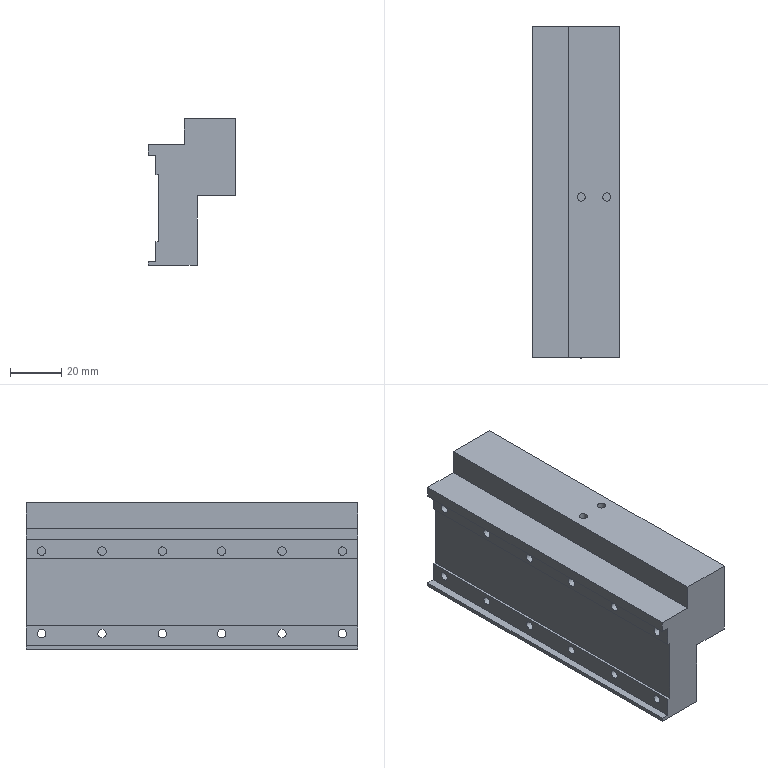CAM job | NX | 3+2 milling, drilling | part box 34 x 129 x 57 mm | stock box 40 x 134 x 60 mm
Tools:
number,name,description,diameter,corner_radius,flute_length,length,flutes
9,D10,平底铣刀-粗,10.0,0.0,35.0,75.0,2
10,D10-J,平底铣刀-精,10.0,0.0,35.0,75.0,2
1,D80R0.8飞刀,圆鼻刀-粗,80.0,0.8,50.0,75.0,2
1,D80R0.8飞刀-J,圆鼻刀-精,80.0,0.8,50.0,75.0,2
2,D6倒角刀,倒角刀,6.0,0.0,3.0,25.0,2
21,M4X0.7,丝锥,3.3,0.0,35.0,50.0,2
17,M6X1.0,丝锥,5.0,0.0,35.0,50.0,2
15,ZT5,钻头,5.0,0.0,35.0,50.0,2
13,钻头3.3,Twist Drill 3.3 mm,3.3,0.0,35.0,35.008,2
Operations:
program,operation,operation_type,tool,method,geometry_group,spindle_rpm,surface_speed,feed_per_tooth,feed_cut,feed_plunge,cut_length_mm,path_length_mm,cut_time_min,machine_time_min
B,底壁铣飞面一刀开粗_COPY,VolumeBased25DMillingOperation,D80R0.8飞刀,分层开粗-切深K-步距G,W-B,5000.0,1256.637,0.3,3000.0,100.0,2609.134,5198.512,0.8697,1.129
B,底壁铣飞面一刀精光_COPY,VolumeBased25DMillingOperation,D80R0.8飞刀-J,侧刃精光-切深K-步距G,W-B,5000.0,1256.637,0.1,1000.0,100.0,236.998,272.998,0.237,0.2406
B,底壁铣分层开粗-中_COPY,VolumeBased25DMillingOperation,D10,分层开粗-切深K-步距G,W-B,8000.0,251.32,0.25,4000.0,100.0,14640.868,15225.158,3.66,3.719
B,打点-深0.8_2,Operation,D6倒角刀,NONE,W-B,8000.0,150.796,0.0312,500.0,90.0,16.2,342.551,0.0324,0.065
B,盲平孔-M6螺纹底孔,Operation,ZT5,NONE,W-B,2800.0,43.982,0.0536,300.0,90.0,39.0,209.023,0.13,0.147
B,钻倒角_2,Operation,D6倒角刀,METHOD,W-B,8000.0,150.796,0.0312,500.0,0.0,31.2,265.358,0.0624,0.0858
B,铣倒角_1,PlanarMilling,D6倒角刀,METHOD,W-B,8000.0,150.796,0.0312,500.0,100.0,58.323,267.728,0.1166,0.1376
B,平面去毛刺6X45L_COPY,SurfaceContour,D6倒角刀,爬面_倒角-切深0-步距G,W-B,6500.0,122.519,0.1154,1500.0,100.0,625.965,1335.941,0.4173,0.4883
B,盲平孔-攻牙M6,Operation,M6X1.0,METHOD,W-B,500.0,7.854,0.001,1.0,90.0,30.0,191.023,30.0,30.016
B,底壁铣精光底面-中_COPY,VolumeBased25DMillingOperation,D10-J,精光步距切深关,W-B,8000.0,251.32,0.0625,1000.0,100.0,861.805,920.405,0.8618,0.8677
B,底壁铣精光侧面-中-选底面_COPY,VolumeBased25DMillingOperation,D10-J,侧刃精光-切深K-步距G,W-B,8000.0,251.32,0.0625,1000.0,100.0,147.681,207.281,0.1477,0.1536
A,顶面,FaceMilling,D80R0.8飞刀,侧刃精光-切深K-步距G,W-A,5000.0,1256.637,0.1,1000.0,100.0,223.0,259.0,0.223,0.2266
A,外形粗_2,VolumeBased25DMillingOperation,D10,METHOD,W-A,8000.0,251.327,0.3125,5000.0,80.0,18183.524,18256.024,3.637,3.644
A,底壁粗_1,VolumeBased25DMillingOperation,D10,METHOD,W-A,6000.0,113.0,0.2083,3500.0,100.0,7904.4,8187.489,2.258,2.287
A,底壁粗_2,VolumeBased25DMillingOperation,D10,METHOD,W-A,6000.0,113.0,0.2083,3500.0,100.0,4376.8,4528.488,1.25,1.266
A,底壁粗_3,VolumeBased25DMillingOperation,D10,METHOD,W-A,6000.0,188.496,0.3333,4000.0,100.0,6660.0,6931.733,1.665,1.692
A,打点-深0.8,Operation,D6倒角刀,NONE,W-A,8000.0,150.796,0.0312,500.0,90.0,21.6,366.529,0.0432,0.0777
A,通孔-M4螺纹底孔,Operation,钻头3.3,NONE,W-A,3000.0,31.102,0.05,300.0,90.0,137.948,444.004,0.4598,0.4904
A,盲平孔-M4螺纹底孔,Operation,钻头3.3,NONE,W-A,3000.0,31.102,0.0417,250.0,90.0,186.0,540.107,0.744,0.7794
A,底精_1,VolumeBased25DMillingOperation,D10-J,METHOD,W-A,6000.0,113.0,0.2083,1200.0,100.0,291.0,358.0,0.2425,0.2492
A,底精_2,VolumeBased25DMillingOperation,D10-J,METHOD,W-A,6000.0,113.0,0.2083,1200.0,100.0,579.099,626.099,0.4826,0.4873
A,仅选体,SurfaceContour,D6倒角刀,METHOD,W-A,8000.0,150.796,0.1875,3000.0,100.0,1100.566,1904.663,0.3669,0.4473
A,钻倒角_1,Operation,D6倒角刀,METHOD,W-A,8000.0,150.796,0.0312,500.0,0.0,62.4,471.955,0.1248,0.1658
A,通孔-攻牙M4,Operation,M4X0.7,METHOD,W-A,600.0,6.22,0.0006,0.7,90.0,120.0,408.107,171.429,171.457
A,底侧精_3,VolumeBased25DMillingOperation,D10-J,METHOD,W-A,6000.0,113.0,0.2083,1200.0,100.0,284.683,544.668,0.2372,0.2632
A,底侧精_4,VolumeBased25DMillingOperation,D10-J,METHOD,W-A,6000.0,113.0,0.2083,1200.0,100.0,284.683,392.563,0.2372,0.248
A,底侧精_5,VolumeBased25DMillingOperation,D10-J,METHOD,W-A,6000.0,113.0,0.2083,1200.0,100.0,284.683,403.783,0.2372,0.2491
A,外形半精_2,VolumeBased25DMillingOperation,D10-J,METHOD,W-A,8000.0,251.327,0.0625,1000.0,100.0,816.748,999.263,0.8167,0.835